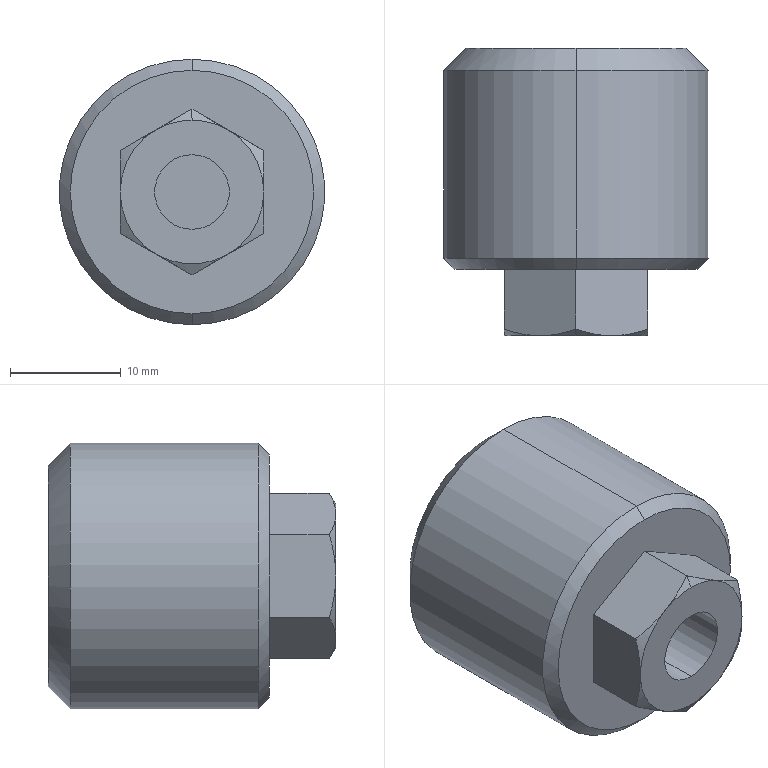Part | 1 solid | 29 faces | box 24 x 26 x 24 mm | volume 9098 mm3 | cone 11 | plane 10 | cylinder 6 | sphere 2 | commonest cylinder face diameters 6.75 x2 8 x2 24 x2
STEP:
#1=CARTESIAN_POINT('',(0.,18.,-4.));
#2=VERTEX_POINT('',#1);
#3=CARTESIAN_POINT('',(0.,18.,4.));
#4=VERTEX_POINT('',#3);
#5=CARTESIAN_POINT('',(0.,18.,0.));
#6=DIRECTION('',(0.,1.,0.));
#7=DIRECTION('',(0.,0.,-1.));
#8=AXIS2_PLACEMENT_3D('',#5,#6,#7);
#9=CIRCLE('',#8,4.);
#10=EDGE_CURVE('',#2,#4,#9,.T.);
#11=ORIENTED_EDGE('',*,*,#10,.T.);
#12=CARTESIAN_POINT('',(0.,14.,0.));
#13=VERTEX_POINT('',#12);
#14=CARTESIAN_POINT('',(0.,18.,0.));
#15=DIRECTION('',(1.,0.,0.));
#16=DIRECTION('',(0.,0.,-1.));
#17=AXIS2_PLACEMENT_3D('',#14,#15,#16);
#18=CIRCLE('',#17,4.);
#19=EDGE_CURVE('',#4,#13,#18,.T.);
#20=ORIENTED_EDGE('',*,*,#19,.T.);
#21=CARTESIAN_POINT('',(0.,18.,0.));
#22=DIRECTION('',(-1.,0.,0.));
#23=DIRECTION('',(0.,0.,1.));
#24=AXIS2_PLACEMENT_3D('',#21,#22,#23);
#25=CIRCLE('',#24,4.);
#26=EDGE_CURVE('',#2,#13,#25,.T.);
#27=ORIENTED_EDGE('',*,*,#26,.F.);
#28=EDGE_LOOP('',(#11,#20,#27));
#29=FACE_OUTER_BOUND('',#28,.T.);
#30=CARTESIAN_POINT('',(0.,18.,0.));
#31=DIRECTION('',(1.,0.,0.));
#32=DIRECTION('',(0.,0.,-1.));
#33=AXIS2_PLACEMENT_3D('',#30,#31,#32);
#34=SPHERICAL_SURFACE('',#33,4.);
#35=ADVANCED_FACE('',(#29),#34,.F.);
#36=CARTESIAN_POINT('',(0.,5.5,3.375));
#37=VERTEX_POINT('',#36);
#38=CARTESIAN_POINT('',(0.,5.5,-3.375));
#39=VERTEX_POINT('',#38);
#40=CARTESIAN_POINT('',(0.,5.5,0.));
#41=DIRECTION('',(0.,-1.,0.));
#42=DIRECTION('',(0.,0.,-1.));
#43=AXIS2_PLACEMENT_3D('',#40,#41,#42);
#44=CIRCLE('',#43,3.375);
#45=EDGE_CURVE('',#37,#39,#44,.T.);
#46=ORIENTED_EDGE('',*,*,#45,.F.);
#47=CARTESIAN_POINT('',(0.,-6.,3.375));
#48=VERTEX_POINT('',#47);
#49=CARTESIAN_POINT('',(0.,5.5,3.375));
#50=DIRECTION('',(0.,-1.,0.));
#51=VECTOR('',#50,1000.);
#52=LINE('',#49,#51);
#53=EDGE_CURVE('',#37,#48,#52,.T.);
#54=ORIENTED_EDGE('',*,*,#53,.T.);
#55=CARTESIAN_POINT('',(0.,-6.,-3.375));
#56=VERTEX_POINT('',#55);
#57=CARTESIAN_POINT('',(0.,-6.,0.));
#58=DIRECTION('',(0.,-1.,0.));
#59=DIRECTION('',(0.,0.,-1.));
#60=AXIS2_PLACEMENT_3D('',#57,#58,#59);
#61=CIRCLE('',#60,3.375);
#62=EDGE_CURVE('',#48,#56,#61,.T.);
#63=ORIENTED_EDGE('',*,*,#62,.T.);
#64=CARTESIAN_POINT('',(0.,5.5,-3.375));
#65=DIRECTION('',(0.,-1.,0.));
#66=VECTOR('',#65,1000.);
#67=LINE('',#64,#66);
#68=EDGE_CURVE('',#39,#56,#67,.T.);
#69=ORIENTED_EDGE('',*,*,#68,.F.);
#70=EDGE_LOOP('',(#46,#54,#63,#69));
#71=FACE_OUTER_BOUND('',#70,.T.);
#72=CARTESIAN_POINT('',(0.,5.5,0.));
#73=DIRECTION('',(0.,-1.,0.));
#74=DIRECTION('',(0.,0.,-1.));
#75=AXIS2_PLACEMENT_3D('',#72,#73,#74);
#76=CYLINDRICAL_SURFACE('',#75,3.375);
#77=ADVANCED_FACE('',(#71),#76,.F.);
#78=ORIENTED_EDGE('',*,*,#10,.F.);
#79=CARTESIAN_POINT('',(0.,20.,-4.));
#80=VERTEX_POINT('',#79);
#81=CARTESIAN_POINT('',(0.,18.,-4.));
#82=DIRECTION('',(0.,1.,0.));
#83=VECTOR('',#82,1000.);
#84=LINE('',#81,#83);
#85=EDGE_CURVE('',#2,#80,#84,.T.);
#86=ORIENTED_EDGE('',*,*,#85,.T.);
#87=CARTESIAN_POINT('',(0.,20.,4.));
#88=VERTEX_POINT('',#87);
#89=CARTESIAN_POINT('',(0.,20.,0.));
#90=DIRECTION('',(0.,-1.,0.));
#91=DIRECTION('',(0.,0.,-1.));
#92=AXIS2_PLACEMENT_3D('',#89,#90,#91);
#93=CIRCLE('',#92,4.);
#94=EDGE_CURVE('',#88,#80,#93,.T.);
#95=ORIENTED_EDGE('',*,*,#94,.F.);
#96=CARTESIAN_POINT('',(0.,18.,4.));
#97=DIRECTION('',(0.,1.,0.));
#98=VECTOR('',#97,1000.);
#99=LINE('',#96,#98);
#100=EDGE_CURVE('',#4,#88,#99,.T.);
#101=ORIENTED_EDGE('',*,*,#100,.F.);
#102=EDGE_LOOP('',(#78,#86,#95,#101));
#103=FACE_OUTER_BOUND('',#102,.T.);
#104=CARTESIAN_POINT('',(0.,18.,0.));
#105=DIRECTION('',(0.,1.,0.));
#106=DIRECTION('',(0.,0.,1.));
#107=AXIS2_PLACEMENT_3D('',#104,#105,#106);
#108=CYLINDRICAL_SURFACE('',#107,4.);
#109=ADVANCED_FACE('',(#103),#108,.F.);
#110=CARTESIAN_POINT('',(-3.25,-6.,5.629));
#111=VERTEX_POINT('',#110);
#112=CARTESIAN_POINT('',(0.,-6.,6.5));
#113=VERTEX_POINT('',#112);
#114=CARTESIAN_POINT('',(0.,-6.,0.));
#115=DIRECTION('',(0.,1.,0.));
#116=DIRECTION('',(0.,0.,1.));
#117=AXIS2_PLACEMENT_3D('',#114,#115,#116);
#118=CIRCLE('',#117,6.5);
#119=EDGE_CURVE('',#111,#113,#118,.T.);
#120=ORIENTED_EDGE('',*,*,#119,.T.);
#121=CARTESIAN_POINT('',(0.,-5.419,7.506));
#122=VERTEX_POINT('',#121);
#123=CARTESIAN_POINT('',(0.,9.65,33.607));
#124=DIRECTION('',(0.,0.5,0.866));
#125=VECTOR('',#124,1000.);
#126=LINE('',#123,#125);
#127=EDGE_CURVE('',#113,#122,#126,.T.);
#128=ORIENTED_EDGE('',*,*,#127,.T.);
#129=CARTESIAN_POINT('',(-3.25,-6.,5.629));
#130=CARTESIAN_POINT('',(-2.982,-6.,5.784));
#131=CARTESIAN_POINT('',(-2.575,-5.98,6.019));
#132=CARTESIAN_POINT('',(-2.093,-5.923,6.297));
#133=CARTESIAN_POINT('',(-1.85,-5.886,6.437));
#134=CARTESIAN_POINT('',(-1.728,-5.865,6.508));
#135=CARTESIAN_POINT('',(-1.676,-5.856,6.538));
#136=CARTESIAN_POINT('',(-1.641,-5.85,6.558));
#137=CARTESIAN_POINT('',(-1.622,-5.846,6.569));
#138=CARTESIAN_POINT('',(-1.099,-5.748,6.871));
#139=CARTESIAN_POINT('',(-0.5631,-5.607,7.18));
#140=CARTESIAN_POINT('',(0.,-5.419,7.506));
#141=B_SPLINE_CURVE_WITH_KNOTS('',3,(#129,#130,#131,#132,#133,#134,#135,#136,#137,#138,#139,#140),.UNSPECIFIED.,.F.,.F.,(4,1,1,1,1,2,2,4),(0.,0.25,0.375,0.4375,0.4687,0.4844,0.5,1.),.UNSPECIFIED.);
#142=EDGE_CURVE('',#111,#122,#141,.T.);
#143=ORIENTED_EDGE('',*,*,#142,.F.);
#144=EDGE_LOOP('',(#120,#128,#143));
#145=FACE_OUTER_BOUND('',#144,.T.);
#146=CARTESIAN_POINT('',(0.,9.65,0.));
#147=DIRECTION('',(0.,1.,0.));
#148=DIRECTION('',(0.,0.,1.));
#149=AXIS2_PLACEMENT_3D('',#146,#147,#148);
#150=CONICAL_SURFACE('',#149,33.607,1.047);
#151=ADVANCED_FACE('',(#145),#150,.T.);
#152=CARTESIAN_POINT('',(0.,0.,-11.));
#153=VERTEX_POINT('',#152);
#154=CARTESIAN_POINT('',(0.,0.,11.));
#155=VERTEX_POINT('',#154);
#156=CARTESIAN_POINT('',(0.,0.,0.));
#157=DIRECTION('',(0.,-1.,0.));
#158=DIRECTION('',(0.,0.,1.));
#159=AXIS2_PLACEMENT_3D('',#156,#157,#158);
#160=CIRCLE('',#159,11.);
#161=EDGE_CURVE('',#153,#155,#160,.T.);
#162=ORIENTED_EDGE('',*,*,#161,.F.);
#163=CARTESIAN_POINT('',(0.,1.,-12.));
#164=VERTEX_POINT('',#163);
#165=CARTESIAN_POINT('',(0.,1.,-12.));
#166=DIRECTION('',(0.,0.7071,-0.7071));
#167=VECTOR('',#166,1000.);
#168=LINE('',#165,#167);
#169=EDGE_CURVE('',#153,#164,#168,.T.);
#170=ORIENTED_EDGE('',*,*,#169,.T.);
#171=CARTESIAN_POINT('',(0.,1.,12.));
#172=VERTEX_POINT('',#171);
#173=CARTESIAN_POINT('',(0.,1.,0.));
#174=DIRECTION('',(0.,1.,0.));
#175=DIRECTION('',(0.,0.,1.));
#176=AXIS2_PLACEMENT_3D('',#173,#174,#175);
#177=CIRCLE('',#176,12.);
#178=EDGE_CURVE('',#172,#164,#177,.T.);
#179=ORIENTED_EDGE('',*,*,#178,.F.);
#180=CARTESIAN_POINT('',(0.,1.,12.));
#181=DIRECTION('',(0.,0.7071,0.7071));
#182=VECTOR('',#181,1000.);
#183=LINE('',#180,#182);
#184=EDGE_CURVE('',#155,#172,#183,.T.);
#185=ORIENTED_EDGE('',*,*,#184,.F.);
#186=EDGE_LOOP('',(#162,#170,#179,#185));
#187=FACE_OUTER_BOUND('',#186,.T.);
#188=CARTESIAN_POINT('',(0.,1.,0.));
#189=DIRECTION('',(0.,1.,0.));
#190=DIRECTION('',(0.,0.,1.));
#191=AXIS2_PLACEMENT_3D('',#188,#189,#190);
#192=CONICAL_SURFACE('',#191,12.,0.7854);
#193=ADVANCED_FACE('',(#187),#192,.T.);
#194=CARTESIAN_POINT('',(0.,20.,10.));
#195=VERTEX_POINT('',#194);
#196=CARTESIAN_POINT('',(0.,20.,-10.));
#197=VERTEX_POINT('',#196);
#198=CARTESIAN_POINT('',(0.,20.,0.));
#199=DIRECTION('',(0.,1.,0.));
#200=DIRECTION('',(0.,0.,1.));
#201=AXIS2_PLACEMENT_3D('',#198,#199,#200);
#202=CIRCLE('',#201,10.);
#203=EDGE_CURVE('',#195,#197,#202,.T.);
#204=ORIENTED_EDGE('',*,*,#203,.F.);
#205=CARTESIAN_POINT('',(0.,18.,12.));
#206=VERTEX_POINT('',#205);
#207=CARTESIAN_POINT('',(0.,18.,12.));
#208=DIRECTION('',(0.,-0.7071,0.7071));
#209=VECTOR('',#208,1000.);
#210=LINE('',#207,#209);
#211=EDGE_CURVE('',#195,#206,#210,.T.);
#212=ORIENTED_EDGE('',*,*,#211,.T.);
#213=CARTESIAN_POINT('',(0.,18.,-12.));
#214=VERTEX_POINT('',#213);
#215=CARTESIAN_POINT('',(0.,18.,0.));
#216=DIRECTION('',(0.,1.,0.));
#217=DIRECTION('',(0.,0.,1.));
#218=AXIS2_PLACEMENT_3D('',#215,#216,#217);
#219=CIRCLE('',#218,12.);
#220=EDGE_CURVE('',#206,#214,#219,.T.);
#221=ORIENTED_EDGE('',*,*,#220,.T.);
#222=CARTESIAN_POINT('',(0.,18.,-12.));
#223=DIRECTION('',(0.,-0.7071,-0.7071));
#224=VECTOR('',#223,1000.);
#225=LINE('',#222,#224);
#226=EDGE_CURVE('',#197,#214,#225,.T.);
#227=ORIENTED_EDGE('',*,*,#226,.F.);
#228=EDGE_LOOP('',(#204,#212,#221,#227));
#229=FACE_OUTER_BOUND('',#228,.T.);
#230=CARTESIAN_POINT('',(0.,18.,0.));
#231=DIRECTION('',(0.,-1.,0.));
#232=DIRECTION('',(0.,0.,-1.));
#233=AXIS2_PLACEMENT_3D('',#230,#231,#232);
#234=CONICAL_SURFACE('',#233,12.,0.7854);
#235=ADVANCED_FACE('',(#229),#234,.T.);
#236=ORIENTED_EDGE('',*,*,#178,.T.);
#237=CARTESIAN_POINT('',(0.,44.545,-12.));
#238=DIRECTION('',(0.,1.,0.));
#239=VECTOR('',#238,1000.);
#240=LINE('',#237,#239);
#241=EDGE_CURVE('',#164,#214,#240,.T.);
#242=ORIENTED_EDGE('',*,*,#241,.T.);
#243=ORIENTED_EDGE('',*,*,#220,.F.);
#244=CARTESIAN_POINT('',(0.,44.545,12.));
#245=DIRECTION('',(0.,1.,0.));
#246=VECTOR('',#245,1000.);
#247=LINE('',#244,#246);
#248=EDGE_CURVE('',#172,#206,#247,.T.);
#249=ORIENTED_EDGE('',*,*,#248,.F.);
#250=EDGE_LOOP('',(#236,#242,#243,#249));
#251=FACE_OUTER_BOUND('',#250,.T.);
#252=CARTESIAN_POINT('',(0.,44.545,0.));
#253=DIRECTION('',(0.,1.,0.));
#254=DIRECTION('',(0.,0.,1.));
#255=AXIS2_PLACEMENT_3D('',#252,#253,#254);
#256=CYLINDRICAL_SURFACE('',#255,12.);
#257=ADVANCED_FACE('',(#251),#256,.T.);
#258=CARTESIAN_POINT('',(0.,0.,7.506));
#259=VERTEX_POINT('',#258);
#260=CARTESIAN_POINT('',(0.,-6.,7.506));
#261=DIRECTION('',(0.,1.,0.));
#262=VECTOR('',#261,1000.);
#263=LINE('',#260,#262);
#264=EDGE_CURVE('',#122,#259,#263,.T.);
#265=ORIENTED_EDGE('',*,*,#264,.F.);
#266=CARTESIAN_POINT('',(3.25,-6.,5.629));
#267=VERTEX_POINT('',#266);
#268=CARTESIAN_POINT('',(0.,-5.419,7.506));
#269=CARTESIAN_POINT('',(0.2818,-5.513,7.343));
#270=CARTESIAN_POINT('',(0.6941,-5.637,7.105));
#271=CARTESIAN_POINT('',(1.157,-5.75,6.837));
#272=CARTESIAN_POINT('',(1.384,-5.8,6.706));
#273=CARTESIAN_POINT('',(1.497,-5.822,6.641));
#274=CARTESIAN_POINT('',(1.545,-5.832,6.614));
#275=CARTESIAN_POINT('',(1.577,-5.838,6.595));
#276=CARTESIAN_POINT('',(1.591,-5.84,6.587));
#277=CARTESIAN_POINT('',(2.167,-5.948,6.255));
#278=CARTESIAN_POINT('',(2.714,-6.,5.939));
#279=CARTESIAN_POINT('',(3.25,-6.,5.629));
#280=B_SPLINE_CURVE_WITH_KNOTS('',3,(#268,#269,#270,#271,#272,#273,#274,#275,#276,#277,#278,#279),.UNSPECIFIED.,.F.,.F.,(4,1,1,1,1,2,2,4),(0.,0.25,0.375,0.4375,0.4688,0.4844,0.5,1.),.UNSPECIFIED.);
#281=EDGE_CURVE('',#122,#267,#280,.T.);
#282=ORIENTED_EDGE('',*,*,#281,.T.);
#283=CARTESIAN_POINT('',(6.5,-5.419,3.753));
#284=VERTEX_POINT('',#283);
#285=CARTESIAN_POINT('',(3.25,-6.,5.629));
#286=CARTESIAN_POINT('',(3.518,-6.,5.474));
#287=CARTESIAN_POINT('',(3.925,-5.98,5.239));
#288=CARTESIAN_POINT('',(4.407,-5.923,4.961));
#289=CARTESIAN_POINT('',(4.65,-5.886,4.821));
#290=CARTESIAN_POINT('',(4.772,-5.865,4.751));
#291=CARTESIAN_POINT('',(4.824,-5.856,4.72));
#292=CARTESIAN_POINT('',(4.859,-5.85,4.7));
#293=CARTESIAN_POINT('',(4.878,-5.846,4.689));
#294=CARTESIAN_POINT('',(5.401,-5.748,4.387));
#295=CARTESIAN_POINT('',(5.937,-5.607,4.078));
#296=CARTESIAN_POINT('',(6.5,-5.419,3.753));
#297=B_SPLINE_CURVE_WITH_KNOTS('',3,(#285,#286,#287,#288,#289,#290,#291,#292,#293,#294,#295,#296),.UNSPECIFIED.,.F.,.F.,(4,1,1,1,1,2,2,4),(0.,0.25,0.375,0.4375,0.4688,0.4844,0.5,1.),.UNSPECIFIED.);
#298=EDGE_CURVE('',#267,#284,#297,.T.);
#299=ORIENTED_EDGE('',*,*,#298,.T.);
#300=CARTESIAN_POINT('',(6.5,0.,3.753));
#301=VERTEX_POINT('',#300);
#302=CARTESIAN_POINT('',(6.5,-6.,3.753));
#303=DIRECTION('',(0.,1.,0.));
#304=VECTOR('',#303,1000.);
#305=LINE('',#302,#304);
#306=EDGE_CURVE('',#284,#301,#305,.T.);
#307=ORIENTED_EDGE('',*,*,#306,.T.);
#308=CARTESIAN_POINT('',(0.,0.,7.506));
#309=DIRECTION('',(0.866,0.,-0.5));
#310=VECTOR('',#309,1000.);
#311=LINE('',#308,#310);
#312=EDGE_CURVE('',#259,#301,#311,.T.);
#313=ORIENTED_EDGE('',*,*,#312,.F.);
#314=EDGE_LOOP('',(#265,#282,#299,#307,#313));
#315=FACE_OUTER_BOUND('',#314,.T.);
#316=CARTESIAN_POINT('',(0.,-6.,7.506));
#317=DIRECTION('',(0.5,0.,0.866));
#318=DIRECTION('',(0.,-1.,0.));
#319=AXIS2_PLACEMENT_3D('',#316,#317,#318);
#320=PLANE('',#319);
#321=ADVANCED_FACE('',(#315),#320,.T.);
#322=CARTESIAN_POINT('',(-6.5,-5.419,3.753));
#323=VERTEX_POINT('',#322);
#324=CARTESIAN_POINT('',(-6.5,0.,3.753));
#325=VERTEX_POINT('',#324);
#326=CARTESIAN_POINT('',(-6.5,-6.,3.753));
#327=DIRECTION('',(0.,1.,0.));
#328=VECTOR('',#327,1000.);
#329=LINE('',#326,#328);
#330=EDGE_CURVE('',#323,#325,#329,.T.);
#331=ORIENTED_EDGE('',*,*,#330,.F.);
#332=CARTESIAN_POINT('',(-6.5,-5.419,3.753));
#333=CARTESIAN_POINT('',(-6.218,-5.513,3.915));
#334=CARTESIAN_POINT('',(-5.806,-5.637,4.154));
#335=CARTESIAN_POINT('',(-5.343,-5.75,4.421));
#336=CARTESIAN_POINT('',(-5.116,-5.8,4.552));
#337=CARTESIAN_POINT('',(-5.003,-5.822,4.617));
#338=CARTESIAN_POINT('',(-4.955,-5.832,4.645));
#339=CARTESIAN_POINT('',(-4.923,-5.838,4.663));
#340=CARTESIAN_POINT('',(-4.909,-5.84,4.671));
#341=CARTESIAN_POINT('',(-4.333,-5.948,5.004));
#342=CARTESIAN_POINT('',(-3.786,-6.,5.32));
#343=CARTESIAN_POINT('',(-3.25,-6.,5.629));
#344=B_SPLINE_CURVE_WITH_KNOTS('',3,(#332,#333,#334,#335,#336,#337,#338,#339,#340,#341,#342,#343),.UNSPECIFIED.,.F.,.F.,(4,1,1,1,1,2,2,4),(0.,0.25,0.375,0.4375,0.4687,0.4844,0.5,1.),.UNSPECIFIED.);
#345=EDGE_CURVE('',#323,#111,#344,.T.);
#346=ORIENTED_EDGE('',*,*,#345,.T.);
#347=ORIENTED_EDGE('',*,*,#142,.T.);
#348=ORIENTED_EDGE('',*,*,#264,.T.);
#349=CARTESIAN_POINT('',(-6.5,0.,3.753));
#350=DIRECTION('',(0.866,0.,0.5));
#351=VECTOR('',#350,1000.);
#352=LINE('',#349,#351);
#353=EDGE_CURVE('',#325,#259,#352,.T.);
#354=ORIENTED_EDGE('',*,*,#353,.F.);
#355=EDGE_LOOP('',(#331,#346,#347,#348,#354));
#356=FACE_OUTER_BOUND('',#355,.T.);
#357=CARTESIAN_POINT('',(-6.5,-6.,3.753));
#358=DIRECTION('',(-0.5,0.,0.866));
#359=DIRECTION('',(0.,1.,0.));
#360=AXIS2_PLACEMENT_3D('',#357,#358,#359);
#361=PLANE('',#360);
#362=ADVANCED_FACE('',(#356),#361,.T.);
#363=CARTESIAN_POINT('',(-6.5,-5.419,-3.753));
#364=VERTEX_POINT('',#363);
#365=CARTESIAN_POINT('',(-6.5,0.,-3.753));
#366=VERTEX_POINT('',#365);
#367=CARTESIAN_POINT('',(-6.5,-6.,-3.753));
#368=DIRECTION('',(0.,1.,0.));
#369=VECTOR('',#368,1000.);
#370=LINE('',#367,#369);
#371=EDGE_CURVE('',#364,#366,#370,.T.);
#372=ORIENTED_EDGE('',*,*,#371,.F.);
#373=CARTESIAN_POINT('',(-6.5,-6.,0.));
#374=VERTEX_POINT('',#373);
#375=CARTESIAN_POINT('',(-6.5,-5.419,-3.753));
#376=CARTESIAN_POINT('',(-6.5,-5.514,-3.427));
#377=CARTESIAN_POINT('',(-6.5,-5.637,-2.949));
#378=CARTESIAN_POINT('',(-6.5,-5.751,-2.413));
#379=CARTESIAN_POINT('',(-6.5,-5.8,-2.151));
#380=CARTESIAN_POINT('',(-6.5,-5.823,-2.02));
#381=CARTESIAN_POINT('',(-6.5,-5.832,-1.965));
#382=CARTESIAN_POINT('',(-6.5,-5.838,-1.928));
#383=CARTESIAN_POINT('',(-6.5,-5.841,-1.911));
#384=CARTESIAN_POINT('',(-6.5,-5.948,-1.248));
#385=CARTESIAN_POINT('',(-6.5,-6.,-0.6178));
#386=CARTESIAN_POINT('',(-6.5,-6.,0.));
#387=B_SPLINE_CURVE_WITH_KNOTS('',3,(#375,#376,#377,#378,#379,#380,#381,#382,#383,#384,#385,#386),.UNSPECIFIED.,.F.,.F.,(4,1,1,1,1,2,2,4),(0.,0.25,0.375,0.4375,0.4687,0.4844,0.5,1.),.UNSPECIFIED.);
#388=EDGE_CURVE('',#364,#374,#387,.T.);
#389=ORIENTED_EDGE('',*,*,#388,.T.);
#390=CARTESIAN_POINT('',(-6.5,-6.,0.));
#391=CARTESIAN_POINT('',(-6.5,-6.,0.3109));
#392=CARTESIAN_POINT('',(-6.5,-5.98,0.7822));
#393=CARTESIAN_POINT('',(-6.5,-5.923,1.341));
#394=CARTESIAN_POINT('',(-6.5,-5.885,1.622));
#395=CARTESIAN_POINT('',(-6.5,-5.864,1.763));
#396=CARTESIAN_POINT('',(-6.5,-5.855,1.824));
#397=CARTESIAN_POINT('',(-6.5,-5.849,1.865));
#398=CARTESIAN_POINT('',(-6.5,-5.845,1.887));
#399=CARTESIAN_POINT('',(-6.5,-5.747,2.489));
#400=CARTESIAN_POINT('',(-6.5,-5.606,3.105));
#401=CARTESIAN_POINT('',(-6.5,-5.419,3.753));
#402=B_SPLINE_CURVE_WITH_KNOTS('',3,(#390,#391,#392,#393,#394,#395,#396,#397,#398,#399,#400,#401),.UNSPECIFIED.,.F.,.F.,(4,1,1,1,1,2,2,4),(0.,0.25,0.375,0.4375,0.4687,0.4844,0.5,1.),.UNSPECIFIED.);
#403=EDGE_CURVE('',#374,#323,#402,.T.);
#404=ORIENTED_EDGE('',*,*,#403,.T.);
#405=ORIENTED_EDGE('',*,*,#330,.T.);
#406=CARTESIAN_POINT('',(-6.5,0.,-3.753));
#407=DIRECTION('',(0.,0.,1.));
#408=VECTOR('',#407,1000.);
#409=LINE('',#406,#408);
#410=EDGE_CURVE('',#366,#325,#409,.T.);
#411=ORIENTED_EDGE('',*,*,#410,.F.);
#412=EDGE_LOOP('',(#372,#389,#404,#405,#411));
#413=FACE_OUTER_BOUND('',#412,.T.);
#414=CARTESIAN_POINT('',(-6.5,-6.,-3.753));
#415=DIRECTION('',(-1.,0.,0.));
#416=DIRECTION('',(0.,0.,1.));
#417=AXIS2_PLACEMENT_3D('',#414,#415,#416);
#418=PLANE('',#417);
#419=ADVANCED_FACE('',(#413),#418,.T.);
#420=CARTESIAN_POINT('',(0.,-5.419,-7.506));
#421=VERTEX_POINT('',#420);
#422=CARTESIAN_POINT('',(0.,0.,-7.506));
#423=VERTEX_POINT('',#422);
#424=CARTESIAN_POINT('',(0.,-6.,-7.506));
#425=DIRECTION('',(0.,1.,0.));
#426=VECTOR('',#425,1000.);
#427=LINE('',#424,#426);
#428=EDGE_CURVE('',#421,#423,#427,.T.);
#429=ORIENTED_EDGE('',*,*,#428,.F.);
#430=CARTESIAN_POINT('',(-3.25,-6.,-5.629));
#431=VERTEX_POINT('',#430);
#432=CARTESIAN_POINT('',(0.,-5.419,-7.506));
#433=CARTESIAN_POINT('',(-0.2818,-5.513,-7.343));
#434=CARTESIAN_POINT('',(-0.6941,-5.637,-7.105));
#435=CARTESIAN_POINT('',(-1.157,-5.75,-6.837));
#436=CARTESIAN_POINT('',(-1.384,-5.8,-6.706));
#437=CARTESIAN_POINT('',(-1.497,-5.822,-6.641));
#438=CARTESIAN_POINT('',(-1.545,-5.832,-6.614));
#439=CARTESIAN_POINT('',(-1.577,-5.838,-6.595));
#440=CARTESIAN_POINT('',(-1.591,-5.84,-6.587));
#441=CARTESIAN_POINT('',(-2.167,-5.948,-6.255));
#442=CARTESIAN_POINT('',(-2.714,-6.,-5.939));
#443=CARTESIAN_POINT('',(-3.25,-6.,-5.629));
#444=B_SPLINE_CURVE_WITH_KNOTS('',3,(#432,#433,#434,#435,#436,#437,#438,#439,#440,#441,#442,#443),.UNSPECIFIED.,.F.,.F.,(4,1,1,1,1,2,2,4),(0.,0.25,0.375,0.4375,0.4687,0.4844,0.5,1.),.UNSPECIFIED.);
#445=EDGE_CURVE('',#421,#431,#444,.T.);
#446=ORIENTED_EDGE('',*,*,#445,.T.);
#447=CARTESIAN_POINT('',(-3.25,-6.,-5.629));
#448=CARTESIAN_POINT('',(-3.518,-6.,-5.474));
#449=CARTESIAN_POINT('',(-3.925,-5.98,-5.239));
#450=CARTESIAN_POINT('',(-4.407,-5.923,-4.961));
#451=CARTESIAN_POINT('',(-4.65,-5.886,-4.821));
#452=CARTESIAN_POINT('',(-4.772,-5.865,-4.751));
#453=CARTESIAN_POINT('',(-4.824,-5.856,-4.72));
#454=CARTESIAN_POINT('',(-4.859,-5.85,-4.7));
#455=CARTESIAN_POINT('',(-4.878,-5.846,-4.689));
#456=CARTESIAN_POINT('',(-5.401,-5.748,-4.387));
#457=CARTESIAN_POINT('',(-5.937,-5.607,-4.078));
#458=CARTESIAN_POINT('',(-6.5,-5.419,-3.753));
#459=B_SPLINE_CURVE_WITH_KNOTS('',3,(#447,#448,#449,#450,#451,#452,#453,#454,#455,#456,#457,#458),.UNSPECIFIED.,.F.,.F.,(4,1,1,1,1,2,2,4),(0.,0.25,0.375,0.4375,0.4687,0.4844,0.5,1.),.UNSPECIFIED.);
#460=EDGE_CURVE('',#431,#364,#459,.T.);
#461=ORIENTED_EDGE('',*,*,#460,.T.);
#462=ORIENTED_EDGE('',*,*,#371,.T.);
#463=CARTESIAN_POINT('',(0.,0.,-7.506));
#464=DIRECTION('',(-0.866,0.,0.5));
#465=VECTOR('',#464,1000.);
#466=LINE('',#463,#465);
#467=EDGE_CURVE('',#423,#366,#466,.T.);
#468=ORIENTED_EDGE('',*,*,#467,.F.);
#469=EDGE_LOOP('',(#429,#446,#461,#462,#468));
#470=FACE_OUTER_BOUND('',#469,.T.);
#471=CARTESIAN_POINT('',(0.,-6.,-7.506));
#472=DIRECTION('',(-0.5,0.,-0.866));
#473=DIRECTION('',(-0.866,0.,0.5));
#474=AXIS2_PLACEMENT_3D('',#471,#472,#473);
#475=PLANE('',#474);
#476=ADVANCED_FACE('',(#470),#475,.T.);
#477=CARTESIAN_POINT('',(6.5,-5.419,-3.753));
#478=VERTEX_POINT('',#477);
#479=CARTESIAN_POINT('',(6.5,0.,-3.753));
#480=VERTEX_POINT('',#479);
#481=CARTESIAN_POINT('',(6.5,-6.,-3.753));
#482=DIRECTION('',(0.,1.,0.));
#483=VECTOR('',#482,1000.);
#484=LINE('',#481,#483);
#485=EDGE_CURVE('',#478,#480,#484,.T.);
#486=ORIENTED_EDGE('',*,*,#485,.F.);
#487=CARTESIAN_POINT('',(3.25,-6.,-5.629));
#488=VERTEX_POINT('',#487);
#489=CARTESIAN_POINT('',(6.5,-5.419,-3.753));
#490=CARTESIAN_POINT('',(6.218,-5.513,-3.915));
#491=CARTESIAN_POINT('',(5.806,-5.637,-4.154));
#492=CARTESIAN_POINT('',(5.343,-5.75,-4.421));
#493=CARTESIAN_POINT('',(5.116,-5.8,-4.552));
#494=CARTESIAN_POINT('',(5.003,-5.822,-4.617));
#495=CARTESIAN_POINT('',(4.955,-5.832,-4.645));
#496=CARTESIAN_POINT('',(4.923,-5.838,-4.663));
#497=CARTESIAN_POINT('',(4.909,-5.84,-4.671));
#498=CARTESIAN_POINT('',(4.333,-5.948,-5.004));
#499=CARTESIAN_POINT('',(3.786,-6.,-5.32));
#500=CARTESIAN_POINT('',(3.25,-6.,-5.629));
#501=B_SPLINE_CURVE_WITH_KNOTS('',3,(#489,#490,#491,#492,#493,#494,#495,#496,#497,#498,#499,#500),.UNSPECIFIED.,.F.,.F.,(4,1,1,1,1,2,2,4),(0.,0.25,0.375,0.4375,0.4688,0.4844,0.5,1.),.UNSPECIFIED.);
#502=EDGE_CURVE('',#478,#488,#501,.T.);
#503=ORIENTED_EDGE('',*,*,#502,.T.);
#504=CARTESIAN_POINT('',(3.25,-6.,-5.629));
#505=CARTESIAN_POINT('',(2.982,-6.,-5.784));
#506=CARTESIAN_POINT('',(2.575,-5.98,-6.019));
#507=CARTESIAN_POINT('',(2.093,-5.923,-6.297));
#508=CARTESIAN_POINT('',(1.85,-5.886,-6.437));
#509=CARTESIAN_POINT('',(1.728,-5.865,-6.508));
#510=CARTESIAN_POINT('',(1.676,-5.856,-6.538));
#511=CARTESIAN_POINT('',(1.641,-5.85,-6.558));
#512=CARTESIAN_POINT('',(1.622,-5.846,-6.569));
#513=CARTESIAN_POINT('',(1.099,-5.748,-6.871));
#514=CARTESIAN_POINT('',(0.5631,-5.607,-7.18));
#515=CARTESIAN_POINT('',(0.,-5.419,-7.506));
#516=B_SPLINE_CURVE_WITH_KNOTS('',3,(#504,#505,#506,#507,#508,#509,#510,#511,#512,#513,#514,#515),.UNSPECIFIED.,.F.,.F.,(4,1,1,1,1,2,2,4),(0.,0.25,0.375,0.4375,0.4687,0.4844,0.5,1.),.UNSPECIFIED.);
#517=EDGE_CURVE('',#488,#421,#516,.T.);
#518=ORIENTED_EDGE('',*,*,#517,.T.);
#519=ORIENTED_EDGE('',*,*,#428,.T.);
#520=CARTESIAN_POINT('',(6.5,0.,-3.753));
#521=DIRECTION('',(-0.866,0.,-0.5));
#522=VECTOR('',#521,1000.);
#523=LINE('',#520,#522);
#524=EDGE_CURVE('',#480,#423,#523,.T.);
#525=ORIENTED_EDGE('',*,*,#524,.F.);
#526=EDGE_LOOP('',(#486,#503,#518,#519,#525));
#527=FACE_OUTER_BOUND('',#526,.T.);
#528=CARTESIAN_POINT('',(6.5,-6.,-3.753));
#529=DIRECTION('',(0.5,0.,-0.866));
#530=DIRECTION('',(0.,-1.,0.));
#531=AXIS2_PLACEMENT_3D('',#528,#529,#530);
#532=PLANE('',#531);
#533=ADVANCED_FACE('',(#527),#532,.T.);
#534=ORIENTED_EDGE('',*,*,#306,.F.);
#535=CARTESIAN_POINT('',(6.5,-6.,0.));
#536=VERTEX_POINT('',#535);
#537=CARTESIAN_POINT('',(6.5,-5.419,3.753));
#538=CARTESIAN_POINT('',(6.5,-5.513,3.429));
#539=CARTESIAN_POINT('',(6.5,-5.636,2.955));
#540=CARTESIAN_POINT('',(6.5,-5.749,2.423));
#541=CARTESIAN_POINT('',(6.5,-5.798,2.163));
#542=CARTESIAN_POINT('',(6.5,-5.821,2.033));
#543=CARTESIAN_POINT('',(6.5,-5.83,1.978));
#544=CARTESIAN_POINT('',(6.5,-5.836,1.942));
#545=CARTESIAN_POINT('',(6.5,-5.839,1.925));
#546=CARTESIAN_POINT('',(6.5,-5.947,1.257));
#547=CARTESIAN_POINT('',(6.5,-6.,0.6221));
#548=CARTESIAN_POINT('',(6.5,-6.,0.));
#549=B_SPLINE_CURVE_WITH_KNOTS('',3,(#537,#538,#539,#540,#541,#542,#543,#544,#545,#546,#547,#548),.UNSPECIFIED.,.F.,.F.,(4,1,1,1,1,2,2,4),(0.,0.25,0.375,0.4375,0.4688,0.4844,0.5,1.),.UNSPECIFIED.);
#550=EDGE_CURVE('',#284,#536,#549,.T.);
#551=ORIENTED_EDGE('',*,*,#550,.T.);
#552=CARTESIAN_POINT('',(6.5,-6.,0.));
#553=CARTESIAN_POINT('',(6.5,-6.,-0.3087));
#554=CARTESIAN_POINT('',(6.5,-5.981,-0.7767));
#555=CARTESIAN_POINT('',(6.5,-5.924,-1.331));
#556=CARTESIAN_POINT('',(6.5,-5.887,-1.61));
#557=CARTESIAN_POINT('',(6.5,-5.866,-1.751));
#558=CARTESIAN_POINT('',(6.5,-5.857,-1.811));
#559=CARTESIAN_POINT('',(6.5,-5.851,-1.851));
#560=CARTESIAN_POINT('',(6.5,-5.847,-1.873));
#561=CARTESIAN_POINT('',(6.5,-5.75,-2.48));
#562=CARTESIAN_POINT('',(6.5,-5.608,-3.1));
#563=CARTESIAN_POINT('',(6.5,-5.419,-3.753));
#564=B_SPLINE_CURVE_WITH_KNOTS('',3,(#552,#553,#554,#555,#556,#557,#558,#559,#560,#561,#562,#563),.UNSPECIFIED.,.F.,.F.,(4,1,1,1,1,2,2,4),(0.,0.25,0.375,0.4375,0.4688,0.4844,0.5,1.),.UNSPECIFIED.);
#565=EDGE_CURVE('',#536,#478,#564,.T.);
#566=ORIENTED_EDGE('',*,*,#565,.T.);
#567=ORIENTED_EDGE('',*,*,#485,.T.);
#568=CARTESIAN_POINT('',(6.5,0.,3.753));
#569=DIRECTION('',(0.,0.,-1.));
#570=VECTOR('',#569,1000.);
#571=LINE('',#568,#570);
#572=EDGE_CURVE('',#301,#480,#571,.T.);
#573=ORIENTED_EDGE('',*,*,#572,.F.);
#574=EDGE_LOOP('',(#534,#551,#566,#567,#573));
#575=FACE_OUTER_BOUND('',#574,.T.);
#576=CARTESIAN_POINT('',(6.5,-6.,3.753));
#577=DIRECTION('',(1.,0.,0.));
#578=DIRECTION('',(0.,0.,-1.));
#579=AXIS2_PLACEMENT_3D('',#576,#577,#578);
#580=PLANE('',#579);
#581=ADVANCED_FACE('',(#575),#580,.T.);
#582=CARTESIAN_POINT('',(0.,0.,0.));
#583=DIRECTION('',(0.,-1.,0.));
#584=DIRECTION('',(0.,0.,1.));
#585=AXIS2_PLACEMENT_3D('',#582,#583,#584);
#586=CIRCLE('',#585,11.);
#587=EDGE_CURVE('',#155,#153,#586,.T.);
#588=ORIENTED_EDGE('',*,*,#587,.T.);
#589=ORIENTED_EDGE('',*,*,#161,.T.);
#590=EDGE_LOOP('',(#588,#589));
#591=FACE_OUTER_BOUND('',#590,.T.);
#592=ORIENTED_EDGE('',*,*,#353,.T.);
#593=ORIENTED_EDGE('',*,*,#312,.T.);
#594=ORIENTED_EDGE('',*,*,#572,.T.);
#595=ORIENTED_EDGE('',*,*,#524,.T.);
#596=ORIENTED_EDGE('',*,*,#467,.T.);
#597=ORIENTED_EDGE('',*,*,#410,.T.);
#598=EDGE_LOOP('',(#592,#593,#594,#595,#596,#597));
#599=FACE_BOUND('',#598,.T.);
#600=CARTESIAN_POINT('',(0.,0.,0.));
#601=DIRECTION('',(0.,1.,0.));
#602=DIRECTION('',(1.,0.,0.));
#603=AXIS2_PLACEMENT_3D('',#600,#601,#602);
#604=PLANE('',#603);
#605=ADVANCED_FACE('',(#591,#599),#604,.F.);
#606=ORIENTED_EDGE('',*,*,#241,.F.);
#607=CARTESIAN_POINT('',(0.,1.,0.));
#608=DIRECTION('',(0.,1.,0.));
#609=DIRECTION('',(0.,0.,1.));
#610=AXIS2_PLACEMENT_3D('',#607,#608,#609);
#611=CIRCLE('',#610,12.);
#612=EDGE_CURVE('',#164,#172,#611,.T.);
#613=ORIENTED_EDGE('',*,*,#612,.T.);
#614=ORIENTED_EDGE('',*,*,#248,.T.);
#615=CARTESIAN_POINT('',(0.,18.,0.));
#616=DIRECTION('',(0.,1.,0.));
#617=DIRECTION('',(0.,0.,1.));
#618=AXIS2_PLACEMENT_3D('',#615,#616,#617);
#619=CIRCLE('',#618,12.);
#620=EDGE_CURVE('',#214,#206,#619,.T.);
#621=ORIENTED_EDGE('',*,*,#620,.F.);
#622=EDGE_LOOP('',(#606,#613,#614,#621));
#623=FACE_OUTER_BOUND('',#622,.T.);
#624=CARTESIAN_POINT('',(0.,44.545,0.));
#625=DIRECTION('',(0.,1.,0.));
#626=DIRECTION('',(0.,0.,1.));
#627=AXIS2_PLACEMENT_3D('',#624,#625,#626);
#628=CYLINDRICAL_SURFACE('',#627,12.);
#629=ADVANCED_FACE('',(#623),#628,.T.);
#630=ORIENTED_EDGE('',*,*,#211,.F.);
#631=CARTESIAN_POINT('',(0.,20.,0.));
#632=DIRECTION('',(0.,1.,0.));
#633=DIRECTION('',(0.,0.,1.));
#634=AXIS2_PLACEMENT_3D('',#631,#632,#633);
#635=CIRCLE('',#634,10.);
#636=EDGE_CURVE('',#197,#195,#635,.T.);
#637=ORIENTED_EDGE('',*,*,#636,.F.);
#638=ORIENTED_EDGE('',*,*,#226,.T.);
#639=ORIENTED_EDGE('',*,*,#620,.T.);
#640=EDGE_LOOP('',(#630,#637,#638,#639));
#641=FACE_OUTER_BOUND('',#640,.T.);
#642=CARTESIAN_POINT('',(0.,18.,0.));
#643=DIRECTION('',(0.,-1.,0.));
#644=DIRECTION('',(0.,0.,-1.));
#645=AXIS2_PLACEMENT_3D('',#642,#643,#644);
#646=CONICAL_SURFACE('',#645,12.,0.7854);
#647=ADVANCED_FACE('',(#641),#646,.T.);
#648=ORIENTED_EDGE('',*,*,#636,.T.);
#649=ORIENTED_EDGE('',*,*,#203,.T.);
#650=EDGE_LOOP('',(#648,#649));
#651=FACE_OUTER_BOUND('',#650,.T.);
#652=ORIENTED_EDGE('',*,*,#94,.T.);
#653=CARTESIAN_POINT('',(0.,20.,0.));
#654=DIRECTION('',(0.,-1.,0.));
#655=DIRECTION('',(0.,0.,-1.));
#656=AXIS2_PLACEMENT_3D('',#653,#654,#655);
#657=CIRCLE('',#656,4.);
#658=EDGE_CURVE('',#80,#88,#657,.T.);
#659=ORIENTED_EDGE('',*,*,#658,.T.);
#660=EDGE_LOOP('',(#652,#659));
#661=FACE_BOUND('',#660,.T.);
#662=CARTESIAN_POINT('',(10.,20.,0.));
#663=DIRECTION('',(0.,-1.,0.));
#664=DIRECTION('',(0.,0.,-1.));
#665=AXIS2_PLACEMENT_3D('',#662,#663,#664);
#666=PLANE('',#665);
#667=ADVANCED_FACE('',(#651,#661),#666,.F.);
#668=ORIENTED_EDGE('',*,*,#169,.F.);
#669=ORIENTED_EDGE('',*,*,#587,.F.);
#670=ORIENTED_EDGE('',*,*,#184,.T.);
#671=ORIENTED_EDGE('',*,*,#612,.F.);
#672=EDGE_LOOP('',(#668,#669,#670,#671));
#673=FACE_OUTER_BOUND('',#672,.T.);
#674=CARTESIAN_POINT('',(0.,1.,0.));
#675=DIRECTION('',(0.,1.,0.));
#676=DIRECTION('',(0.,0.,1.));
#677=AXIS2_PLACEMENT_3D('',#674,#675,#676);
#678=CONICAL_SURFACE('',#677,12.,0.7854);
#679=ADVANCED_FACE('',(#673),#678,.T.);
#680=ORIENTED_EDGE('',*,*,#127,.F.);
#681=CARTESIAN_POINT('',(0.,-6.,0.));
#682=DIRECTION('',(0.,1.,0.));
#683=DIRECTION('',(0.,0.,1.));
#684=AXIS2_PLACEMENT_3D('',#681,#682,#683);
#685=CIRCLE('',#684,6.5);
#686=EDGE_CURVE('',#113,#267,#685,.T.);
#687=ORIENTED_EDGE('',*,*,#686,.T.);
#688=ORIENTED_EDGE('',*,*,#281,.F.);
#689=EDGE_LOOP('',(#680,#687,#688));
#690=FACE_OUTER_BOUND('',#689,.T.);
#691=CARTESIAN_POINT('',(0.,9.65,0.));
#692=DIRECTION('',(0.,1.,0.));
#693=DIRECTION('',(0.,0.,1.));
#694=AXIS2_PLACEMENT_3D('',#691,#692,#693);
#695=CONICAL_SURFACE('',#694,33.607,1.047);
#696=ADVANCED_FACE('',(#690),#695,.T.);
#697=CARTESIAN_POINT('',(0.,-6.,0.));
#698=DIRECTION('',(0.,1.,0.));
#699=DIRECTION('',(0.,0.,1.));
#700=AXIS2_PLACEMENT_3D('',#697,#698,#699);
#701=CIRCLE('',#700,6.5);
#702=EDGE_CURVE('',#374,#111,#701,.T.);
#703=ORIENTED_EDGE('',*,*,#702,.T.);
#704=ORIENTED_EDGE('',*,*,#345,.F.);
#705=ORIENTED_EDGE('',*,*,#403,.F.);
#706=EDGE_LOOP('',(#703,#704,#705));
#707=FACE_OUTER_BOUND('',#706,.T.);
#708=CARTESIAN_POINT('',(0.,9.65,0.));
#709=DIRECTION('',(0.,1.,0.));
#710=DIRECTION('',(0.,0.,1.));
#711=AXIS2_PLACEMENT_3D('',#708,#709,#710);
#712=CONICAL_SURFACE('',#711,33.607,1.047);
#713=ADVANCED_FACE('',(#707),#712,.T.);
#714=ORIENTED_EDGE('',*,*,#460,.F.);
#715=CARTESIAN_POINT('',(0.,-6.,0.));
#716=DIRECTION('',(0.,1.,0.));
#717=DIRECTION('',(0.,0.,1.));
#718=AXIS2_PLACEMENT_3D('',#715,#716,#717);
#719=CIRCLE('',#718,6.5);
#720=EDGE_CURVE('',#431,#374,#719,.T.);
#721=ORIENTED_EDGE('',*,*,#720,.T.);
#722=ORIENTED_EDGE('',*,*,#388,.F.);
#723=EDGE_LOOP('',(#714,#721,#722));
#724=FACE_OUTER_BOUND('',#723,.T.);
#725=CARTESIAN_POINT('',(0.,9.65,0.));
#726=DIRECTION('',(0.,1.,0.));
#727=DIRECTION('',(0.,0.,1.));
#728=AXIS2_PLACEMENT_3D('',#725,#726,#727);
#729=CONICAL_SURFACE('',#728,33.607,1.047);
#730=ADVANCED_FACE('',(#724),#729,.T.);
#731=ORIENTED_EDGE('',*,*,#517,.F.);
#732=CARTESIAN_POINT('',(0.,-6.,0.));
#733=DIRECTION('',(0.,1.,0.));
#734=DIRECTION('',(0.,0.,1.));
#735=AXIS2_PLACEMENT_3D('',#732,#733,#734);
#736=CIRCLE('',#735,6.5);
#737=EDGE_CURVE('',#488,#431,#736,.T.);
#738=ORIENTED_EDGE('',*,*,#737,.T.);
#739=ORIENTED_EDGE('',*,*,#445,.F.);
#740=EDGE_LOOP('',(#731,#738,#739));
#741=FACE_OUTER_BOUND('',#740,.T.);
#742=CARTESIAN_POINT('',(0.,9.65,0.));
#743=DIRECTION('',(0.,1.,0.));
#744=DIRECTION('',(0.,0.,1.));
#745=AXIS2_PLACEMENT_3D('',#742,#743,#744);
#746=CONICAL_SURFACE('',#745,33.607,1.047);
#747=ADVANCED_FACE('',(#741),#746,.T.);
#748=ORIENTED_EDGE('',*,*,#565,.F.);
#749=CARTESIAN_POINT('',(0.,-6.,0.));
#750=DIRECTION('',(0.,1.,0.));
#751=DIRECTION('',(0.,0.,1.));
#752=AXIS2_PLACEMENT_3D('',#749,#750,#751);
#753=CIRCLE('',#752,6.5);
#754=EDGE_CURVE('',#536,#488,#753,.T.);
#755=ORIENTED_EDGE('',*,*,#754,.T.);
#756=ORIENTED_EDGE('',*,*,#502,.F.);
#757=EDGE_LOOP('',(#748,#755,#756));
#758=FACE_OUTER_BOUND('',#757,.T.);
#759=CARTESIAN_POINT('',(0.,9.65,0.));
#760=DIRECTION('',(0.,1.,0.));
#761=DIRECTION('',(0.,0.,1.));
#762=AXIS2_PLACEMENT_3D('',#759,#760,#761);
#763=CONICAL_SURFACE('',#762,33.607,1.047);
#764=ADVANCED_FACE('',(#758),#763,.T.);
#765=CARTESIAN_POINT('',(0.,-6.,0.));
#766=DIRECTION('',(0.,1.,0.));
#767=DIRECTION('',(0.,0.,1.));
#768=AXIS2_PLACEMENT_3D('',#765,#766,#767);
#769=CIRCLE('',#768,6.5);
#770=EDGE_CURVE('',#267,#536,#769,.T.);
#771=ORIENTED_EDGE('',*,*,#770,.T.);
#772=ORIENTED_EDGE('',*,*,#550,.F.);
#773=ORIENTED_EDGE('',*,*,#298,.F.);
#774=EDGE_LOOP('',(#771,#772,#773));
#775=FACE_OUTER_BOUND('',#774,.T.);
#776=CARTESIAN_POINT('',(0.,9.65,0.));
#777=DIRECTION('',(0.,1.,0.));
#778=DIRECTION('',(0.,0.,1.));
#779=AXIS2_PLACEMENT_3D('',#776,#777,#778);
#780=CONICAL_SURFACE('',#779,33.607,1.047);
#781=ADVANCED_FACE('',(#775),#780,.T.);
#782=ORIENTED_EDGE('',*,*,#770,.F.);
#783=ORIENTED_EDGE('',*,*,#686,.F.);
#784=ORIENTED_EDGE('',*,*,#119,.F.);
#785=ORIENTED_EDGE('',*,*,#702,.F.);
#786=ORIENTED_EDGE('',*,*,#720,.F.);
#787=ORIENTED_EDGE('',*,*,#737,.F.);
#788=ORIENTED_EDGE('',*,*,#754,.F.);
#789=EDGE_LOOP('',(#782,#783,#784,#785,#786,#787,#788));
#790=FACE_OUTER_BOUND('',#789,.T.);
#791=CARTESIAN_POINT('',(0.,-6.,0.));
#792=DIRECTION('',(0.,-1.,0.));
#793=DIRECTION('',(0.,0.,-1.));
#794=AXIS2_PLACEMENT_3D('',#791,#792,#793);
#795=CIRCLE('',#794,3.375);
#796=EDGE_CURVE('',#56,#48,#795,.T.);
#797=ORIENTED_EDGE('',*,*,#796,.F.);
#798=ORIENTED_EDGE('',*,*,#62,.F.);
#799=EDGE_LOOP('',(#797,#798));
#800=FACE_BOUND('',#799,.T.);
#801=CARTESIAN_POINT('',(0.,-6.,0.));
#802=DIRECTION('',(0.,1.,0.));
#803=DIRECTION('',(1.,0.,0.));
#804=AXIS2_PLACEMENT_3D('',#801,#802,#803);
#805=PLANE('',#804);
#806=ADVANCED_FACE('',(#790,#800),#805,.F.);
#807=ORIENTED_EDGE('',*,*,#85,.F.);
#808=CARTESIAN_POINT('',(0.,18.,0.));
#809=DIRECTION('',(0.,1.,0.));
#810=DIRECTION('',(0.,0.,-1.));
#811=AXIS2_PLACEMENT_3D('',#808,#809,#810);
#812=CIRCLE('',#811,4.);
#813=EDGE_CURVE('',#4,#2,#812,.T.);
#814=ORIENTED_EDGE('',*,*,#813,.F.);
#815=ORIENTED_EDGE('',*,*,#100,.T.);
#816=ORIENTED_EDGE('',*,*,#658,.F.);
#817=EDGE_LOOP('',(#807,#814,#815,#816));
#818=FACE_OUTER_BOUND('',#817,.T.);
#819=CARTESIAN_POINT('',(0.,18.,0.));
#820=DIRECTION('',(0.,1.,0.));
#821=DIRECTION('',(0.,0.,1.));
#822=AXIS2_PLACEMENT_3D('',#819,#820,#821);
#823=CYLINDRICAL_SURFACE('',#822,4.);
#824=ADVANCED_FACE('',(#818),#823,.F.);
#825=ORIENTED_EDGE('',*,*,#19,.F.);
#826=ORIENTED_EDGE('',*,*,#813,.T.);
#827=ORIENTED_EDGE('',*,*,#26,.T.);
#828=EDGE_LOOP('',(#825,#826,#827));
#829=FACE_OUTER_BOUND('',#828,.T.);
#830=CARTESIAN_POINT('',(0.,18.,0.));
#831=DIRECTION('',(1.,0.,0.));
#832=DIRECTION('',(0.,0.,-1.));
#833=AXIS2_PLACEMENT_3D('',#830,#831,#832);
#834=SPHERICAL_SURFACE('',#833,4.);
#835=ADVANCED_FACE('',(#829),#834,.F.);
#836=ORIENTED_EDGE('',*,*,#53,.F.);
#837=CARTESIAN_POINT('',(0.,5.5,0.));
#838=DIRECTION('',(0.,-1.,0.));
#839=DIRECTION('',(0.,0.,-1.));
#840=AXIS2_PLACEMENT_3D('',#837,#838,#839);
#841=CIRCLE('',#840,3.375);
#842=EDGE_CURVE('',#39,#37,#841,.T.);
#843=ORIENTED_EDGE('',*,*,#842,.F.);
#844=ORIENTED_EDGE('',*,*,#68,.T.);
#845=ORIENTED_EDGE('',*,*,#796,.T.);
#846=EDGE_LOOP('',(#836,#843,#844,#845));
#847=FACE_OUTER_BOUND('',#846,.T.);
#848=CARTESIAN_POINT('',(0.,5.5,0.));
#849=DIRECTION('',(0.,-1.,0.));
#850=DIRECTION('',(0.,0.,-1.));
#851=AXIS2_PLACEMENT_3D('',#848,#849,#850);
#852=CYLINDRICAL_SURFACE('',#851,3.375);
#853=ADVANCED_FACE('',(#847),#852,.F.);
#854=ORIENTED_EDGE('',*,*,#842,.T.);
#855=ORIENTED_EDGE('',*,*,#45,.T.);
#856=EDGE_LOOP('',(#854,#855));
#857=FACE_OUTER_BOUND('',#856,.T.);
#858=CARTESIAN_POINT('',(0.,5.5,0.));
#859=DIRECTION('',(0.,-1.,0.));
#860=DIRECTION('',(0.,0.,-1.));
#861=AXIS2_PLACEMENT_3D('',#858,#859,#860);
#862=PLANE('',#861);
#863=ADVANCED_FACE('',(#857),#862,.T.);
#864=CLOSED_SHELL('',(#35,#77,#109,#151,#193,#235,#257,#321,#362,#419,#476,#533,#581,#605,#629,#647,#667,#679,#696,#713,#730,#747,#764,#781,#806,#824,#835,#853,#863));
#865=MANIFOLD_SOLID_BREP('',#864);
#866=CARTESIAN_POINT('',(0.,0.,0.));
#867=DIRECTION('',(0.,0.,1.));
#868=DIRECTION('',(1.,0.,0.));
#869=AXIS2_PLACEMENT_3D('',#866,#867,#868);
#870=(LENGTH_UNIT()NAMED_UNIT(*)SI_UNIT(.MILLI.,.METRE.));
#871=UNCERTAINTY_MEASURE_WITH_UNIT(LENGTH_MEASURE(0.00001),#870,'','');
#872=(NAMED_UNIT(*)PLANE_ANGLE_UNIT()SI_UNIT($,.RADIAN.));
#873=(NAMED_UNIT(*)SI_UNIT($,.STERADIAN.)SOLID_ANGLE_UNIT());
#874=(GEOMETRIC_REPRESENTATION_CONTEXT(3)GLOBAL_UNCERTAINTY_ASSIGNED_CONTEXT((#871))GLOBAL_UNIT_ASSIGNED_CONTEXT((#870,#872,#873))REPRESENTATION_CONTEXT('',''));
#875=ADVANCED_BREP_SHAPE_REPRESENTATION('',(#865,#869),#874);